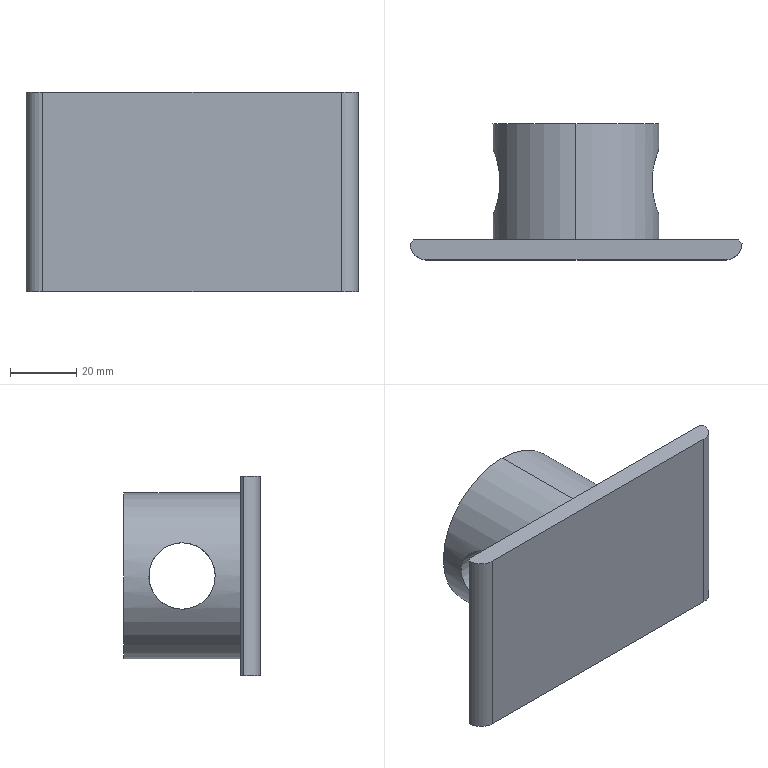Part | SolidWorks | features ICE 2, Chamfer 1, Extrusion 1, Fillet 1 | 1 solid | 13 faces | box 100 x 41 x 60 mm | volume 88631 mm3 | plane 7 | cylinder 6 | commonest cylinder face diameters 10 x2 20 x2 50 x2
STEP:
#1=CARTESIAN_POINT('',(-22.913,17.5,10.));
#2=VERTEX_POINT('',#1);
#3=CARTESIAN_POINT('',(-22.913,17.5,-10.));
#4=VERTEX_POINT('',#3);
#5=CARTESIAN_POINT('',(-22.913,17.5,10.));
#6=CARTESIAN_POINT('',(-22.913,17.171,10.));
#7=CARTESIAN_POINT('',(-22.92,16.842,9.984));
#8=CARTESIAN_POINT('',(-22.948,16.184,9.918));
#9=CARTESIAN_POINT('',(-22.97,15.852,9.869));
#10=CARTESIAN_POINT('',(-23.053,14.881,9.674));
#11=CARTESIAN_POINT('',(-23.134,14.256,9.482));
#12=CARTESIAN_POINT('',(-23.284,13.35,9.104));
#13=CARTESIAN_POINT('',(-23.339,13.051,8.962));
#14=CARTESIAN_POINT('',(-23.456,12.476,8.652));
#15=CARTESIAN_POINT('',(-23.517,12.198,8.485));
#16=CARTESIAN_POINT('',(-23.707,11.392,7.944));
#17=CARTESIAN_POINT('',(-23.843,10.89,7.532));
#18=CARTESIAN_POINT('',(-24.115,9.968,6.61));
#19=CARTESIAN_POINT('',(-24.248,9.558,6.111));
#20=CARTESIAN_POINT('',(-24.432,9.018,5.306));
#21=CARTESIAN_POINT('',(-24.491,8.85,5.028));
#22=CARTESIAN_POINT('',(-24.602,8.54,4.452));
#23=CARTESIAN_POINT('',(-24.655,8.397,4.153));
#24=CARTESIAN_POINT('',(-24.796,8.019,3.247));
#25=CARTESIAN_POINT('',(-24.87,7.828,2.623));
#26=CARTESIAN_POINT('',(-24.947,7.633,1.656));
#27=CARTESIAN_POINT('',(-24.967,7.583,1.327));
#28=CARTESIAN_POINT('',(-24.993,7.517,0.6643));
#29=CARTESIAN_POINT('',(-25.,7.5,0.3339));
#30=CARTESIAN_POINT('',(-25.,7.5,-0.6544));
#31=CARTESIAN_POINT('',(-24.974,7.564,-1.31));
#32=CARTESIAN_POINT('',(-24.897,7.759,-2.287));
#33=CARTESIAN_POINT('',(-24.866,7.841,-2.609));
#34=CARTESIAN_POINT('',(-24.792,8.033,-3.237));
#35=CARTESIAN_POINT('',(-24.749,8.143,-3.544));
#36=CARTESIAN_POINT('',(-24.656,8.394,-4.147));
#37=CARTESIAN_POINT('',(-24.604,8.535,-4.442));
#38=CARTESIAN_POINT('',(-24.493,8.844,-5.019));
#39=CARTESIAN_POINT('',(-24.433,9.014,-5.301));
#40=CARTESIAN_POINT('',(-24.248,9.558,-6.111));
#41=CARTESIAN_POINT('',(-24.115,9.968,-6.609));
#42=CARTESIAN_POINT('',(-23.912,10.655,-7.298));
#43=CARTESIAN_POINT('',(-23.844,10.898,-7.518));
#44=CARTESIAN_POINT('',(-23.71,11.4,-7.931));
#45=CARTESIAN_POINT('',(-23.644,11.659,-8.124));
#46=CARTESIAN_POINT('',(-23.454,12.464,-8.664));
#47=CARTESIAN_POINT('',(-23.336,13.034,-8.972));
#48=CARTESIAN_POINT('',(-23.185,13.946,-9.353));
#49=CARTESIAN_POINT('',(-23.139,14.256,-9.465));
#50=CARTESIAN_POINT('',(-23.06,14.883,-9.657));
#51=CARTESIAN_POINT('',(-23.026,15.201,-9.738));
#52=CARTESIAN_POINT('',(-22.97,15.845,-9.867));
#53=CARTESIAN_POINT('',(-22.949,16.171,-9.917));
#54=CARTESIAN_POINT('',(-22.92,16.831,-9.983));
#55=CARTESIAN_POINT('',(-22.913,17.166,-10.));
#56=CARTESIAN_POINT('',(-22.913,17.5,-10.));
#57=B_SPLINE_CURVE_WITH_KNOTS('',3,(#5,#6,#7,#8,#9,#10,#11,#12,#13,#14,#15,#16,#17,#18,#19,#20,#21,#22,#23,#24,#25,#26,#27,#28,#29,#30,#31,#32,#33,#34,#35,#36,#37,#38,#39,#40,#41,#42,#43,#44,#45,#46,#47,#48,#49,#50,#51,#52,#53,#54,#55,#56),.UNSPECIFIED.,.F.,.F.,(4,2,2,2,2,2,2,2,2,2,2,2,2,2,2,2,2,2,2,2,2,2,2,2,2,4),(0.0316,0.03258,0.03357,0.03554,0.03653,0.03752,0.03949,0.04146,0.04245,0.04344,0.04541,0.04639,0.04738,0.04935,0.05034,0.05133,0.05231,0.0533,0.05527,0.05626,0.05725,0.05922,0.06021,0.06119,0.06218,0.06317),.UNSPECIFIED.);
#58=EDGE_CURVE('',#2,#4,#57,.T.);
#59=ORIENTED_EDGE('',*,*,#58,.F.);
#60=CARTESIAN_POINT('',(22.913,17.5,10.));
#61=VERTEX_POINT('',#60);
#62=CARTESIAN_POINT('',(-50.,17.5,10.));
#63=DIRECTION('',(1.,0.,0.));
#64=VECTOR('',#63,1000.);
#65=LINE('',#62,#64);
#66=EDGE_CURVE('',#2,#61,#65,.T.);
#67=ORIENTED_EDGE('',*,*,#66,.T.);
#68=CARTESIAN_POINT('',(22.913,17.5,-10.));
#69=VERTEX_POINT('',#68);
#70=CARTESIAN_POINT('',(22.913,17.5,-10.));
#71=CARTESIAN_POINT('',(22.913,16.832,-10.));
#72=CARTESIAN_POINT('',(22.942,16.176,-9.934));
#73=CARTESIAN_POINT('',(23.025,15.21,-9.74));
#74=CARTESIAN_POINT('',(23.059,14.892,-9.659));
#75=CARTESIAN_POINT('',(23.139,14.26,-9.466));
#76=CARTESIAN_POINT('',(23.185,13.948,-9.354));
#77=CARTESIAN_POINT('',(23.335,13.043,-8.976));
#78=CARTESIAN_POINT('',(23.452,12.472,-8.668));
#79=CARTESIAN_POINT('',(23.644,11.661,-8.125));
#80=CARTESIAN_POINT('',(23.71,11.397,-7.929));
#81=CARTESIAN_POINT('',(23.844,10.896,-7.516));
#82=CARTESIAN_POINT('',(23.912,10.657,-7.299));
#83=CARTESIAN_POINT('',(24.114,9.972,-6.615));
#84=CARTESIAN_POINT('',(24.247,9.559,-6.113));
#85=CARTESIAN_POINT('',(24.496,8.83,-5.026));
#86=CARTESIAN_POINT('',(24.608,8.523,-4.454));
#87=CARTESIAN_POINT('',(24.748,8.147,-3.553));
#88=CARTESIAN_POINT('',(24.791,8.035,-3.245));
#89=CARTESIAN_POINT('',(24.865,7.842,-2.615));
#90=CARTESIAN_POINT('',(24.897,7.76,-2.291));
#91=CARTESIAN_POINT('',(24.974,7.565,-1.32));
#92=CARTESIAN_POINT('',(25.,7.5,-0.6657));
#93=CARTESIAN_POINT('',(25.,7.5,0.3251));
#94=CARTESIAN_POINT('',(24.994,7.516,0.6588));
#95=CARTESIAN_POINT('',(24.967,7.582,1.321));
#96=CARTESIAN_POINT('',(24.948,7.631,1.648));
#97=CARTESIAN_POINT('',(24.871,7.826,2.615));
#98=CARTESIAN_POINT('',(24.796,8.017,3.243));
#99=CARTESIAN_POINT('',(24.606,8.527,4.463));
#100=CARTESIAN_POINT('',(24.494,8.836,5.036));
#101=CARTESIAN_POINT('',(24.309,9.378,5.843));
#102=CARTESIAN_POINT('',(24.245,9.572,6.104));
#103=CARTESIAN_POINT('',(24.112,9.987,6.608));
#104=CARTESIAN_POINT('',(24.045,10.207,6.849));
#105=CARTESIAN_POINT('',(23.842,10.894,7.535));
#106=CARTESIAN_POINT('',(23.707,11.392,7.945));
#107=CARTESIAN_POINT('',(23.516,12.202,8.488));
#108=CARTESIAN_POINT('',(23.454,12.484,8.657));
#109=CARTESIAN_POINT('',(23.337,13.06,8.966));
#110=CARTESIAN_POINT('',(23.283,13.354,9.106));
#111=CARTESIAN_POINT('',(23.134,14.255,9.481));
#112=CARTESIAN_POINT('',(23.053,14.879,9.673));
#113=CARTESIAN_POINT('',(22.969,15.856,9.87));
#114=CARTESIAN_POINT('',(22.948,16.186,9.919));
#115=CARTESIAN_POINT('',(22.92,16.842,9.984));
#116=CARTESIAN_POINT('',(22.913,17.171,10.));
#117=CARTESIAN_POINT('',(22.913,17.5,10.));
#118=B_SPLINE_CURVE_WITH_KNOTS('',3,(#70,#71,#72,#73,#74,#75,#76,#77,#78,#79,#80,#81,#82,#83,#84,#85,#86,#87,#88,#89,#90,#91,#92,#93,#94,#95,#96,#97,#98,#99,#100,#101,#102,#103,#104,#105,#106,#107,#108,#109,#110,#111,#112,#113,#114,#115,#116,#117),.UNSPECIFIED.,.F.,.F.,(4,2,2,2,2,2,2,2,2,2,2,2,2,2,2,2,2,2,2,2,2,2,2,4),(0.,0.001975,0.002962,0.00395,0.005924,0.006912,0.007899,0.009874,0.01185,0.01284,0.01382,0.0158,0.01679,0.01777,0.01975,0.02172,0.02271,0.0237,0.02567,0.02666,0.02765,0.02962,0.03061,0.0316),.UNSPECIFIED.);
#119=EDGE_CURVE('',#69,#61,#118,.T.);
#120=ORIENTED_EDGE('',*,*,#119,.F.);
#121=CARTESIAN_POINT('',(-50.,17.5,-10.));
#122=DIRECTION('',(1.,0.,0.));
#123=VECTOR('',#122,1000.);
#124=LINE('',#121,#123);
#125=EDGE_CURVE('',#4,#69,#124,.T.);
#126=ORIENTED_EDGE('',*,*,#125,.F.);
#127=EDGE_LOOP('',(#59,#67,#120,#126));
#128=FACE_OUTER_BOUND('',#127,.T.);
#129=CARTESIAN_POINT('',(-50.,17.5,0.));
#130=DIRECTION('',(1.,0.,0.));
#131=DIRECTION('',(0.,0.,-1.));
#132=AXIS2_PLACEMENT_3D('',#129,#130,#131);
#133=CYLINDRICAL_SURFACE('',#132,10.);
#134=ADVANCED_FACE('',(#128),#133,.F.);
#135=ORIENTED_EDGE('',*,*,#119,.T.);
#136=CARTESIAN_POINT('',(22.913,17.5,10.));
#137=CARTESIAN_POINT('',(22.913,17.829,10.));
#138=CARTESIAN_POINT('',(22.92,18.158,9.984));
#139=CARTESIAN_POINT('',(22.948,18.816,9.918));
#140=CARTESIAN_POINT('',(22.97,19.148,9.869));
#141=CARTESIAN_POINT('',(23.053,20.119,9.674));
#142=CARTESIAN_POINT('',(23.134,20.744,9.482));
#143=CARTESIAN_POINT('',(23.284,21.65,9.104));
#144=CARTESIAN_POINT('',(23.339,21.949,8.962));
#145=CARTESIAN_POINT('',(23.456,22.524,8.652));
#146=CARTESIAN_POINT('',(23.517,22.802,8.485));
#147=CARTESIAN_POINT('',(23.707,23.608,7.944));
#148=CARTESIAN_POINT('',(23.843,24.11,7.532));
#149=CARTESIAN_POINT('',(24.115,25.032,6.61));
#150=CARTESIAN_POINT('',(24.248,25.442,6.111));
#151=CARTESIAN_POINT('',(24.432,25.982,5.306));
#152=CARTESIAN_POINT('',(24.491,26.15,5.028));
#153=CARTESIAN_POINT('',(24.602,26.46,4.452));
#154=CARTESIAN_POINT('',(24.655,26.603,4.153));
#155=CARTESIAN_POINT('',(24.796,26.981,3.247));
#156=CARTESIAN_POINT('',(24.87,27.172,2.623));
#157=CARTESIAN_POINT('',(24.947,27.367,1.656));
#158=CARTESIAN_POINT('',(24.967,27.417,1.327));
#159=CARTESIAN_POINT('',(24.993,27.483,0.6643));
#160=CARTESIAN_POINT('',(25.,27.5,0.3339));
#161=CARTESIAN_POINT('',(25.,27.5,-0.6544));
#162=CARTESIAN_POINT('',(24.974,27.436,-1.31));
#163=CARTESIAN_POINT('',(24.897,27.241,-2.287));
#164=CARTESIAN_POINT('',(24.866,27.159,-2.609));
#165=CARTESIAN_POINT('',(24.792,26.967,-3.237));
#166=CARTESIAN_POINT('',(24.749,26.857,-3.544));
#167=CARTESIAN_POINT('',(24.656,26.606,-4.147));
#168=CARTESIAN_POINT('',(24.604,26.465,-4.442));
#169=CARTESIAN_POINT('',(24.493,26.156,-5.019));
#170=CARTESIAN_POINT('',(24.433,25.986,-5.301));
#171=CARTESIAN_POINT('',(24.248,25.442,-6.111));
#172=CARTESIAN_POINT('',(24.115,25.032,-6.609));
#173=CARTESIAN_POINT('',(23.912,24.345,-7.298));
#174=CARTESIAN_POINT('',(23.844,24.102,-7.518));
#175=CARTESIAN_POINT('',(23.71,23.6,-7.931));
#176=CARTESIAN_POINT('',(23.644,23.341,-8.124));
#177=CARTESIAN_POINT('',(23.454,22.536,-8.664));
#178=CARTESIAN_POINT('',(23.336,21.966,-8.972));
#179=CARTESIAN_POINT('',(23.185,21.054,-9.353));
#180=CARTESIAN_POINT('',(23.139,20.744,-9.465));
#181=CARTESIAN_POINT('',(23.06,20.117,-9.657));
#182=CARTESIAN_POINT('',(23.026,19.799,-9.738));
#183=CARTESIAN_POINT('',(22.97,19.155,-9.867));
#184=CARTESIAN_POINT('',(22.949,18.829,-9.917));
#185=CARTESIAN_POINT('',(22.92,18.169,-9.983));
#186=CARTESIAN_POINT('',(22.913,17.834,-10.));
#187=CARTESIAN_POINT('',(22.913,17.5,-10.));
#188=B_SPLINE_CURVE_WITH_KNOTS('',3,(#136,#137,#138,#139,#140,#141,#142,#143,#144,#145,#146,#147,#148,#149,#150,#151,#152,#153,#154,#155,#156,#157,#158,#159,#160,#161,#162,#163,#164,#165,#166,#167,#168,#169,#170,#171,#172,#173,#174,#175,#176,#177,#178,#179,#180,#181,#182,#183,#184,#185,#186,#187),.UNSPECIFIED.,.F.,.F.,(4,2,2,2,2,2,2,2,2,2,2,2,2,2,2,2,2,2,2,2,2,2,2,2,2,4),(0.0316,0.03258,0.03357,0.03554,0.03653,0.03752,0.03949,0.04146,0.04245,0.04344,0.04541,0.04639,0.04738,0.04935,0.05034,0.05133,0.05231,0.0533,0.05527,0.05626,0.05725,0.05922,0.06021,0.06119,0.06218,0.06317),.UNSPECIFIED.);
#189=EDGE_CURVE('',#61,#69,#188,.T.);
#190=ORIENTED_EDGE('',*,*,#189,.T.);
#191=EDGE_LOOP('',(#135,#190));
#192=FACE_BOUND('',#191,.T.);
#193=CARTESIAN_POINT('',(0.,35.,25.));
#194=VERTEX_POINT('',#193);
#195=CARTESIAN_POINT('',(0.,35.,-25.));
#196=VERTEX_POINT('',#195);
#197=CARTESIAN_POINT('',(0.,35.,0.));
#198=DIRECTION('',(0.,1.,0.));
#199=DIRECTION('',(0.,0.,1.));
#200=AXIS2_PLACEMENT_3D('',#197,#198,#199);
#201=CIRCLE('',#200,25.);
#202=EDGE_CURVE('',#194,#196,#201,.T.);
#203=ORIENTED_EDGE('',*,*,#202,.F.);
#204=CARTESIAN_POINT('',(0.,0.,25.));
#205=VERTEX_POINT('',#204);
#206=CARTESIAN_POINT('',(0.,35.,25.));
#207=DIRECTION('',(0.,-1.,0.));
#208=VECTOR('',#207,1000.);
#209=LINE('',#206,#208);
#210=EDGE_CURVE('',#194,#205,#209,.T.);
#211=ORIENTED_EDGE('',*,*,#210,.T.);
#212=CARTESIAN_POINT('',(0.,0.,-25.));
#213=VERTEX_POINT('',#212);
#214=CARTESIAN_POINT('',(0.,0.,0.));
#215=DIRECTION('',(0.,1.,0.));
#216=DIRECTION('',(0.,0.,1.));
#217=AXIS2_PLACEMENT_3D('',#214,#215,#216);
#218=CIRCLE('',#217,25.);
#219=EDGE_CURVE('',#205,#213,#218,.T.);
#220=ORIENTED_EDGE('',*,*,#219,.T.);
#221=CARTESIAN_POINT('',(0.,35.,-25.));
#222=DIRECTION('',(0.,-1.,0.));
#223=VECTOR('',#222,1000.);
#224=LINE('',#221,#223);
#225=EDGE_CURVE('',#196,#213,#224,.T.);
#226=ORIENTED_EDGE('',*,*,#225,.F.);
#227=EDGE_LOOP('',(#203,#211,#220,#226));
#228=FACE_OUTER_BOUND('',#227,.T.);
#229=CARTESIAN_POINT('',(0.,35.,0.));
#230=DIRECTION('',(0.,-1.,0.));
#231=DIRECTION('',(0.,0.,-1.));
#232=AXIS2_PLACEMENT_3D('',#229,#230,#231);
#233=CYLINDRICAL_SURFACE('',#232,25.);
#234=ADVANCED_FACE('',(#192,#228),#233,.T.);
#235=ORIENTED_EDGE('',*,*,#210,.F.);
#236=CARTESIAN_POINT('',(0.,35.,0.));
#237=DIRECTION('',(0.,1.,0.));
#238=DIRECTION('',(0.,0.,1.));
#239=AXIS2_PLACEMENT_3D('',#236,#237,#238);
#240=CIRCLE('',#239,25.);
#241=EDGE_CURVE('',#196,#194,#240,.T.);
#242=ORIENTED_EDGE('',*,*,#241,.F.);
#243=ORIENTED_EDGE('',*,*,#225,.T.);
#244=CARTESIAN_POINT('',(0.,0.,0.));
#245=DIRECTION('',(0.,1.,0.));
#246=DIRECTION('',(0.,0.,1.));
#247=AXIS2_PLACEMENT_3D('',#244,#245,#246);
#248=CIRCLE('',#247,25.);
#249=EDGE_CURVE('',#213,#205,#248,.T.);
#250=ORIENTED_EDGE('',*,*,#249,.T.);
#251=EDGE_LOOP('',(#235,#242,#243,#250));
#252=FACE_OUTER_BOUND('',#251,.T.);
#253=CARTESIAN_POINT('',(-22.913,17.5,-10.));
#254=CARTESIAN_POINT('',(-22.913,18.168,-10.));
#255=CARTESIAN_POINT('',(-22.942,18.824,-9.934));
#256=CARTESIAN_POINT('',(-23.025,19.79,-9.74));
#257=CARTESIAN_POINT('',(-23.059,20.108,-9.659));
#258=CARTESIAN_POINT('',(-23.139,20.74,-9.466));
#259=CARTESIAN_POINT('',(-23.185,21.052,-9.354));
#260=CARTESIAN_POINT('',(-23.335,21.957,-8.976));
#261=CARTESIAN_POINT('',(-23.452,22.528,-8.668));
#262=CARTESIAN_POINT('',(-23.644,23.339,-8.125));
#263=CARTESIAN_POINT('',(-23.71,23.603,-7.929));
#264=CARTESIAN_POINT('',(-23.844,24.104,-7.516));
#265=CARTESIAN_POINT('',(-23.912,24.343,-7.299));
#266=CARTESIAN_POINT('',(-24.114,25.028,-6.615));
#267=CARTESIAN_POINT('',(-24.247,25.441,-6.113));
#268=CARTESIAN_POINT('',(-24.496,26.17,-5.026));
#269=CARTESIAN_POINT('',(-24.608,26.477,-4.454));
#270=CARTESIAN_POINT('',(-24.748,26.853,-3.553));
#271=CARTESIAN_POINT('',(-24.791,26.965,-3.245));
#272=CARTESIAN_POINT('',(-24.865,27.158,-2.615));
#273=CARTESIAN_POINT('',(-24.897,27.24,-2.291));
#274=CARTESIAN_POINT('',(-24.974,27.435,-1.32));
#275=CARTESIAN_POINT('',(-25.,27.5,-0.6657));
#276=CARTESIAN_POINT('',(-25.,27.5,0.3251));
#277=CARTESIAN_POINT('',(-24.994,27.484,0.6588));
#278=CARTESIAN_POINT('',(-24.967,27.418,1.321));
#279=CARTESIAN_POINT('',(-24.948,27.369,1.648));
#280=CARTESIAN_POINT('',(-24.871,27.174,2.615));
#281=CARTESIAN_POINT('',(-24.796,26.983,3.243));
#282=CARTESIAN_POINT('',(-24.606,26.473,4.463));
#283=CARTESIAN_POINT('',(-24.494,26.164,5.036));
#284=CARTESIAN_POINT('',(-24.309,25.622,5.843));
#285=CARTESIAN_POINT('',(-24.245,25.428,6.104));
#286=CARTESIAN_POINT('',(-24.112,25.013,6.608));
#287=CARTESIAN_POINT('',(-24.045,24.793,6.849));
#288=CARTESIAN_POINT('',(-23.842,24.106,7.535));
#289=CARTESIAN_POINT('',(-23.707,23.608,7.945));
#290=CARTESIAN_POINT('',(-23.516,22.798,8.488));
#291=CARTESIAN_POINT('',(-23.454,22.516,8.657));
#292=CARTESIAN_POINT('',(-23.337,21.94,8.966));
#293=CARTESIAN_POINT('',(-23.283,21.646,9.106));
#294=CARTESIAN_POINT('',(-23.134,20.745,9.481));
#295=CARTESIAN_POINT('',(-23.053,20.121,9.673));
#296=CARTESIAN_POINT('',(-22.969,19.144,9.87));
#297=CARTESIAN_POINT('',(-22.948,18.814,9.919));
#298=CARTESIAN_POINT('',(-22.92,18.158,9.984));
#299=CARTESIAN_POINT('',(-22.913,17.829,10.));
#300=CARTESIAN_POINT('',(-22.913,17.5,10.));
#301=B_SPLINE_CURVE_WITH_KNOTS('',3,(#253,#254,#255,#256,#257,#258,#259,#260,#261,#262,#263,#264,#265,#266,#267,#268,#269,#270,#271,#272,#273,#274,#275,#276,#277,#278,#279,#280,#281,#282,#283,#284,#285,#286,#287,#288,#289,#290,#291,#292,#293,#294,#295,#296,#297,#298,#299,#300),.UNSPECIFIED.,.F.,.F.,(4,2,2,2,2,2,2,2,2,2,2,2,2,2,2,2,2,2,2,2,2,2,2,4),(0.,0.001975,0.002962,0.00395,0.005924,0.006912,0.007899,0.009874,0.01185,0.01284,0.01382,0.0158,0.01679,0.01777,0.01975,0.02172,0.02271,0.0237,0.02567,0.02666,0.02765,0.02962,0.03061,0.0316),.UNSPECIFIED.);
#302=EDGE_CURVE('',#4,#2,#301,.T.);
#303=ORIENTED_EDGE('',*,*,#302,.T.);
#304=ORIENTED_EDGE('',*,*,#58,.T.);
#305=EDGE_LOOP('',(#303,#304));
#306=FACE_BOUND('',#305,.T.);
#307=CARTESIAN_POINT('',(0.,35.,0.));
#308=DIRECTION('',(0.,-1.,0.));
#309=DIRECTION('',(0.,0.,-1.));
#310=AXIS2_PLACEMENT_3D('',#307,#308,#309);
#311=CYLINDRICAL_SURFACE('',#310,25.);
#312=ADVANCED_FACE('',(#252,#306),#311,.T.);
#313=ORIENTED_EDGE('',*,*,#241,.T.);
#314=ORIENTED_EDGE('',*,*,#202,.T.);
#315=EDGE_LOOP('',(#313,#314));
#316=FACE_OUTER_BOUND('',#315,.T.);
#317=CARTESIAN_POINT('',(0.,35.,0.));
#318=DIRECTION('',(0.,1.,0.));
#319=DIRECTION('',(0.,0.,1.));
#320=AXIS2_PLACEMENT_3D('',#317,#318,#319);
#321=PLANE('',#320);
#322=ADVANCED_FACE('',(#316),#321,.T.);
#323=CARTESIAN_POINT('',(49.,0.,30.));
#324=VERTEX_POINT('',#323);
#325=CARTESIAN_POINT('',(-49.,0.,30.));
#326=VERTEX_POINT('',#325);
#327=CARTESIAN_POINT('',(-50.,0.,30.));
#328=DIRECTION('',(-1.,0.,0.));
#329=VECTOR('',#328,1000.);
#330=LINE('',#327,#329);
#331=EDGE_CURVE('',#324,#326,#330,.T.);
#332=ORIENTED_EDGE('',*,*,#331,.T.);
#333=CARTESIAN_POINT('',(-50.,-1.,30.));
#334=VERTEX_POINT('',#333);
#335=CARTESIAN_POINT('',(-50.,-1.,30.));
#336=DIRECTION('',(-0.7071,-0.7071,0.));
#337=VECTOR('',#336,1000.);
#338=LINE('',#335,#337);
#339=EDGE_CURVE('',#326,#334,#338,.T.);
#340=ORIENTED_EDGE('',*,*,#339,.T.);
#341=CARTESIAN_POINT('',(-45.,-6.,30.));
#342=VERTEX_POINT('',#341);
#343=CARTESIAN_POINT('',(-45.,-1.,30.));
#344=DIRECTION('',(0.,0.,1.));
#345=DIRECTION('',(-1.,0.,0.));
#346=AXIS2_PLACEMENT_3D('',#343,#344,#345);
#347=CIRCLE('',#346,5.);
#348=EDGE_CURVE('',#334,#342,#347,.T.);
#349=ORIENTED_EDGE('',*,*,#348,.T.);
#350=CARTESIAN_POINT('',(45.,-6.,30.));
#351=VERTEX_POINT('',#350);
#352=CARTESIAN_POINT('',(-50.,-6.,30.));
#353=DIRECTION('',(-1.,0.,0.));
#354=VECTOR('',#353,1000.);
#355=LINE('',#352,#354);
#356=EDGE_CURVE('',#351,#342,#355,.T.);
#357=ORIENTED_EDGE('',*,*,#356,.F.);
#358=CARTESIAN_POINT('',(50.,-1.,30.));
#359=VERTEX_POINT('',#358);
#360=CARTESIAN_POINT('',(45.,-1.,30.));
#361=DIRECTION('',(0.,0.,1.));
#362=DIRECTION('',(-1.,0.,0.));
#363=AXIS2_PLACEMENT_3D('',#360,#361,#362);
#364=CIRCLE('',#363,5.);
#365=EDGE_CURVE('',#351,#359,#364,.T.);
#366=ORIENTED_EDGE('',*,*,#365,.T.);
#367=CARTESIAN_POINT('',(50.,-1.,30.));
#368=DIRECTION('',(-0.7071,0.7071,0.));
#369=VECTOR('',#368,1000.);
#370=LINE('',#367,#369);
#371=EDGE_CURVE('',#359,#324,#370,.T.);
#372=ORIENTED_EDGE('',*,*,#371,.T.);
#373=EDGE_LOOP('',(#332,#340,#349,#357,#366,#372));
#374=FACE_OUTER_BOUND('',#373,.T.);
#375=CARTESIAN_POINT('',(-50.,-6.,30.));
#376=DIRECTION('',(0.,0.,-1.));
#377=DIRECTION('',(-1.,0.,0.));
#378=AXIS2_PLACEMENT_3D('',#375,#376,#377);
#379=PLANE('',#378);
#380=ADVANCED_FACE('',(#374),#379,.F.);
#381=CARTESIAN_POINT('',(-45.,-6.,-30.));
#382=VERTEX_POINT('',#381);
#383=CARTESIAN_POINT('',(-50.,-1.,-30.));
#384=VERTEX_POINT('',#383);
#385=CARTESIAN_POINT('',(-45.,-1.,-30.));
#386=DIRECTION('',(0.,0.,-1.));
#387=DIRECTION('',(1.,0.,0.));
#388=AXIS2_PLACEMENT_3D('',#385,#386,#387);
#389=CIRCLE('',#388,5.);
#390=EDGE_CURVE('',#382,#384,#389,.T.);
#391=ORIENTED_EDGE('',*,*,#390,.T.);
#392=CARTESIAN_POINT('',(-49.,0.,-30.));
#393=VERTEX_POINT('',#392);
#394=CARTESIAN_POINT('',(-50.,-1.,-30.));
#395=DIRECTION('',(0.7071,0.7071,0.));
#396=VECTOR('',#395,1000.);
#397=LINE('',#394,#396);
#398=EDGE_CURVE('',#384,#393,#397,.T.);
#399=ORIENTED_EDGE('',*,*,#398,.T.);
#400=CARTESIAN_POINT('',(49.,0.,-30.));
#401=VERTEX_POINT('',#400);
#402=CARTESIAN_POINT('',(-50.,0.,-30.));
#403=DIRECTION('',(1.,0.,0.));
#404=VECTOR('',#403,1000.);
#405=LINE('',#402,#404);
#406=EDGE_CURVE('',#393,#401,#405,.T.);
#407=ORIENTED_EDGE('',*,*,#406,.T.);
#408=CARTESIAN_POINT('',(50.,-1.,-30.));
#409=VERTEX_POINT('',#408);
#410=CARTESIAN_POINT('',(50.,-1.,-30.));
#411=DIRECTION('',(0.7071,-0.7071,0.));
#412=VECTOR('',#411,1000.);
#413=LINE('',#410,#412);
#414=EDGE_CURVE('',#401,#409,#413,.T.);
#415=ORIENTED_EDGE('',*,*,#414,.T.);
#416=CARTESIAN_POINT('',(45.,-6.,-30.));
#417=VERTEX_POINT('',#416);
#418=CARTESIAN_POINT('',(45.,-1.,-30.));
#419=DIRECTION('',(0.,0.,-1.));
#420=DIRECTION('',(1.,0.,0.));
#421=AXIS2_PLACEMENT_3D('',#418,#419,#420);
#422=CIRCLE('',#421,5.);
#423=EDGE_CURVE('',#409,#417,#422,.T.);
#424=ORIENTED_EDGE('',*,*,#423,.T.);
#425=CARTESIAN_POINT('',(-50.,-6.,-30.));
#426=DIRECTION('',(1.,0.,0.));
#427=VECTOR('',#426,1000.);
#428=LINE('',#425,#427);
#429=EDGE_CURVE('',#382,#417,#428,.T.);
#430=ORIENTED_EDGE('',*,*,#429,.F.);
#431=EDGE_LOOP('',(#391,#399,#407,#415,#424,#430));
#432=FACE_OUTER_BOUND('',#431,.T.);
#433=CARTESIAN_POINT('',(-50.,-6.,-30.));
#434=DIRECTION('',(0.,0.,1.));
#435=DIRECTION('',(1.,0.,0.));
#436=AXIS2_PLACEMENT_3D('',#433,#434,#435);
#437=PLANE('',#436);
#438=ADVANCED_FACE('',(#432),#437,.F.);
#439=ORIENTED_EDGE('',*,*,#356,.T.);
#440=CARTESIAN_POINT('',(-45.,-6.,0.));
#441=DIRECTION('',(0.,0.,-1.));
#442=VECTOR('',#441,1000.);
#443=LINE('',#440,#442);
#444=EDGE_CURVE('',#342,#382,#443,.T.);
#445=ORIENTED_EDGE('',*,*,#444,.T.);
#446=ORIENTED_EDGE('',*,*,#429,.T.);
#447=CARTESIAN_POINT('',(45.,-6.,0.));
#448=DIRECTION('',(0.,0.,1.));
#449=VECTOR('',#448,1000.);
#450=LINE('',#447,#449);
#451=EDGE_CURVE('',#417,#351,#450,.T.);
#452=ORIENTED_EDGE('',*,*,#451,.T.);
#453=EDGE_LOOP('',(#439,#445,#446,#452));
#454=FACE_OUTER_BOUND('',#453,.T.);
#455=CARTESIAN_POINT('',(0.,-6.,0.));
#456=DIRECTION('',(0.,1.,0.));
#457=DIRECTION('',(0.,0.,1.));
#458=AXIS2_PLACEMENT_3D('',#455,#456,#457);
#459=PLANE('',#458);
#460=ADVANCED_FACE('',(#454),#459,.F.);
#461=ORIENTED_EDGE('',*,*,#249,.F.);
#462=ORIENTED_EDGE('',*,*,#219,.F.);
#463=EDGE_LOOP('',(#461,#462));
#464=FACE_BOUND('',#463,.T.);
#465=ORIENTED_EDGE('',*,*,#406,.F.);
#466=CARTESIAN_POINT('',(-49.,0.,30.));
#467=DIRECTION('',(0.,0.,1.));
#468=VECTOR('',#467,1000.);
#469=LINE('',#466,#468);
#470=EDGE_CURVE('',#393,#326,#469,.T.);
#471=ORIENTED_EDGE('',*,*,#470,.T.);
#472=ORIENTED_EDGE('',*,*,#331,.F.);
#473=CARTESIAN_POINT('',(49.,0.,-30.));
#474=DIRECTION('',(0.,0.,-1.));
#475=VECTOR('',#474,1000.);
#476=LINE('',#473,#475);
#477=EDGE_CURVE('',#324,#401,#476,.T.);
#478=ORIENTED_EDGE('',*,*,#477,.T.);
#479=EDGE_LOOP('',(#465,#471,#472,#478));
#480=FACE_OUTER_BOUND('',#479,.T.);
#481=CARTESIAN_POINT('',(0.,0.,0.));
#482=DIRECTION('',(0.,1.,0.));
#483=DIRECTION('',(0.,0.,1.));
#484=AXIS2_PLACEMENT_3D('',#481,#482,#483);
#485=PLANE('',#484);
#486=ADVANCED_FACE('',(#464,#480),#485,.T.);
#487=ORIENTED_EDGE('',*,*,#66,.F.);
#488=ORIENTED_EDGE('',*,*,#302,.F.);
#489=ORIENTED_EDGE('',*,*,#125,.T.);
#490=ORIENTED_EDGE('',*,*,#189,.F.);
#491=EDGE_LOOP('',(#487,#488,#489,#490));
#492=FACE_OUTER_BOUND('',#491,.T.);
#493=CARTESIAN_POINT('',(-50.,17.5,0.));
#494=DIRECTION('',(1.,0.,0.));
#495=DIRECTION('',(0.,0.,-1.));
#496=AXIS2_PLACEMENT_3D('',#493,#494,#495);
#497=CYLINDRICAL_SURFACE('',#496,10.);
#498=ADVANCED_FACE('',(#492),#497,.F.);
#499=ORIENTED_EDGE('',*,*,#348,.F.);
#500=CARTESIAN_POINT('',(-50.,-1.,-30.));
#501=DIRECTION('',(0.,0.,1.));
#502=VECTOR('',#501,1000.);
#503=LINE('',#500,#502);
#504=EDGE_CURVE('',#384,#334,#503,.T.);
#505=ORIENTED_EDGE('',*,*,#504,.F.);
#506=ORIENTED_EDGE('',*,*,#390,.F.);
#507=ORIENTED_EDGE('',*,*,#444,.F.);
#508=EDGE_LOOP('',(#499,#505,#506,#507));
#509=FACE_OUTER_BOUND('',#508,.T.);
#510=CARTESIAN_POINT('',(-45.,-1.,0.));
#511=DIRECTION('',(0.,0.,-1.));
#512=DIRECTION('',(-1.,0.,0.));
#513=AXIS2_PLACEMENT_3D('',#510,#511,#512);
#514=CYLINDRICAL_SURFACE('',#513,5.);
#515=ADVANCED_FACE('',(#509),#514,.T.);
#516=ORIENTED_EDGE('',*,*,#423,.F.);
#517=CARTESIAN_POINT('',(50.,-1.,-30.));
#518=DIRECTION('',(0.,0.,-1.));
#519=VECTOR('',#518,1000.);
#520=LINE('',#517,#519);
#521=EDGE_CURVE('',#359,#409,#520,.T.);
#522=ORIENTED_EDGE('',*,*,#521,.F.);
#523=ORIENTED_EDGE('',*,*,#365,.F.);
#524=ORIENTED_EDGE('',*,*,#451,.F.);
#525=EDGE_LOOP('',(#516,#522,#523,#524));
#526=FACE_OUTER_BOUND('',#525,.T.);
#527=CARTESIAN_POINT('',(45.,-1.,0.));
#528=DIRECTION('',(0.,0.,1.));
#529=DIRECTION('',(1.,0.,0.));
#530=AXIS2_PLACEMENT_3D('',#527,#528,#529);
#531=CYLINDRICAL_SURFACE('',#530,5.);
#532=ADVANCED_FACE('',(#526),#531,.T.);
#533=ORIENTED_EDGE('',*,*,#339,.F.);
#534=ORIENTED_EDGE('',*,*,#470,.F.);
#535=ORIENTED_EDGE('',*,*,#398,.F.);
#536=ORIENTED_EDGE('',*,*,#504,.T.);
#537=EDGE_LOOP('',(#533,#534,#535,#536));
#538=FACE_OUTER_BOUND('',#537,.T.);
#539=CARTESIAN_POINT('',(-50.,-1.,-30.));
#540=DIRECTION('',(-0.7071,0.7071,0.));
#541=DIRECTION('',(0.,0.,1.));
#542=AXIS2_PLACEMENT_3D('',#539,#540,#541);
#543=PLANE('',#542);
#544=ADVANCED_FACE('',(#538),#543,.T.);
#545=ORIENTED_EDGE('',*,*,#414,.F.);
#546=ORIENTED_EDGE('',*,*,#477,.F.);
#547=ORIENTED_EDGE('',*,*,#371,.F.);
#548=ORIENTED_EDGE('',*,*,#521,.T.);
#549=EDGE_LOOP('',(#545,#546,#547,#548));
#550=FACE_OUTER_BOUND('',#549,.T.);
#551=CARTESIAN_POINT('',(50.,-1.,-30.));
#552=DIRECTION('',(0.7071,0.7071,0.));
#553=DIRECTION('',(0.,0.,-1.));
#554=AXIS2_PLACEMENT_3D('',#551,#552,#553);
#555=PLANE('',#554);
#556=ADVANCED_FACE('',(#550),#555,.T.);
#557=CLOSED_SHELL('',(#134,#234,#312,#322,#380,#438,#460,#486,#498,#515,#532,#544,#556));
#558=MANIFOLD_SOLID_BREP('',#557);
#559=CARTESIAN_POINT('',(0.,0.,0.));
#560=DIRECTION('',(0.,0.,1.));
#561=DIRECTION('',(1.,0.,0.));
#562=AXIS2_PLACEMENT_3D('',#559,#560,#561);
#563=(LENGTH_UNIT()NAMED_UNIT(*)SI_UNIT(.MILLI.,.METRE.));
#564=UNCERTAINTY_MEASURE_WITH_UNIT(LENGTH_MEASURE(0.00001),#563,'','');
#565=(NAMED_UNIT(*)PLANE_ANGLE_UNIT()SI_UNIT($,.RADIAN.));
#566=(NAMED_UNIT(*)SI_UNIT($,.STERADIAN.)SOLID_ANGLE_UNIT());
#567=(GEOMETRIC_REPRESENTATION_CONTEXT(3)GLOBAL_UNCERTAINTY_ASSIGNED_CONTEXT((#564))GLOBAL_UNIT_ASSIGNED_CONTEXT((#563,#565,#566))REPRESENTATION_CONTEXT('',''));
#568=ADVANCED_BREP_SHAPE_REPRESENTATION('',(#558,#562),#567);